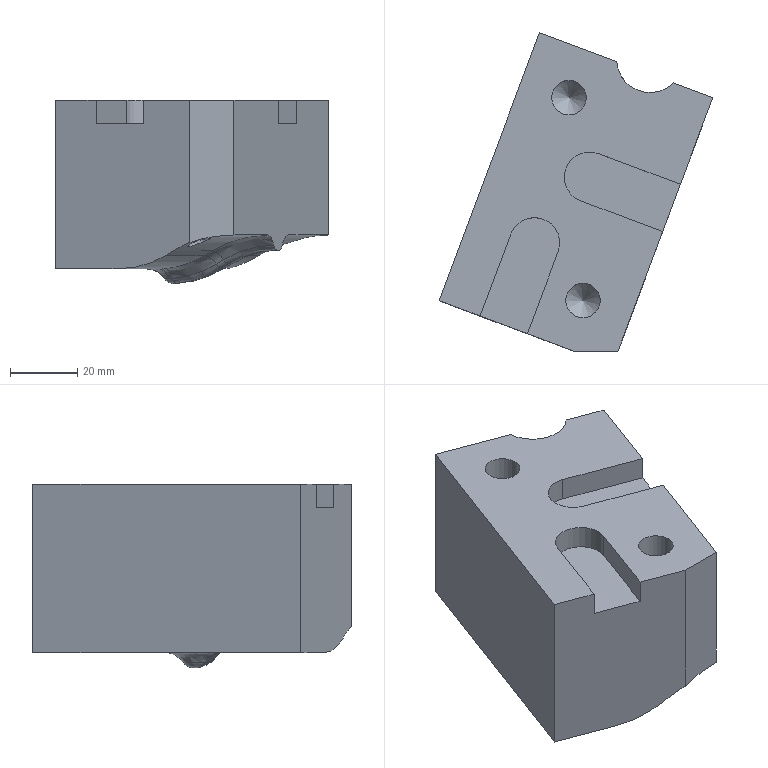Part | NX | features 8 2 | 1 solid | 50 faces | box 81.284 x 94.59 x 54.47 mm | volume 205000 mm3 | plane 17 | cylinder 17 | spline 11 | cone 4 | torus 1 | commonest cylinder face diameters 6 x2 6.8 x2 10.3 x2 13 x2 15 x2 60 x2